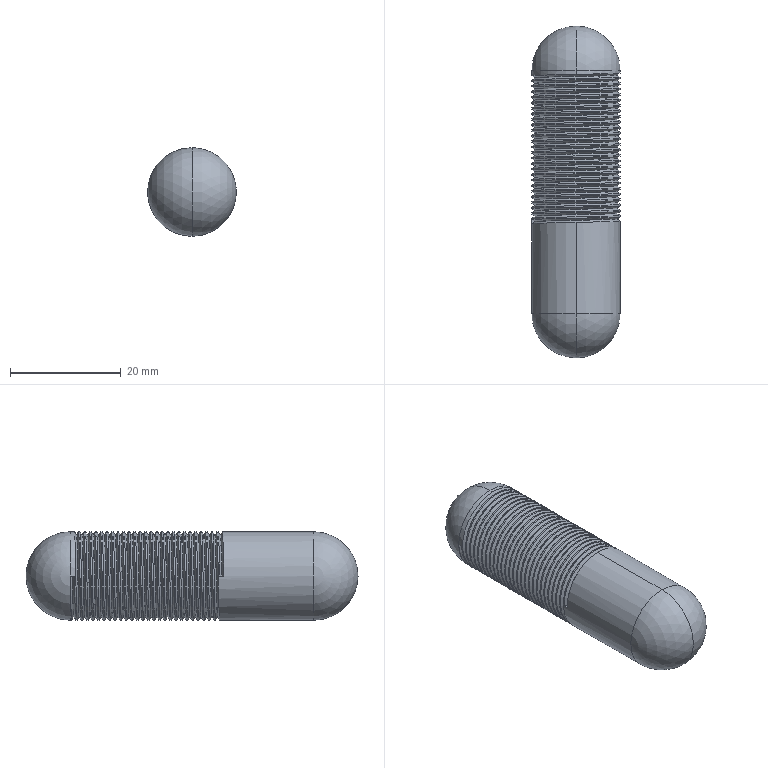Part | SolidWorks | features Fillet 2, Revolution 1, SweepThread 1 | 1 solid | 65 faces | box 16 x 60 x 16 mm | volume 10676 mm3 | cylinder 56 | sphere 4 | spline 3 | plane 2 | commonest cylinder face diameters 16 x56